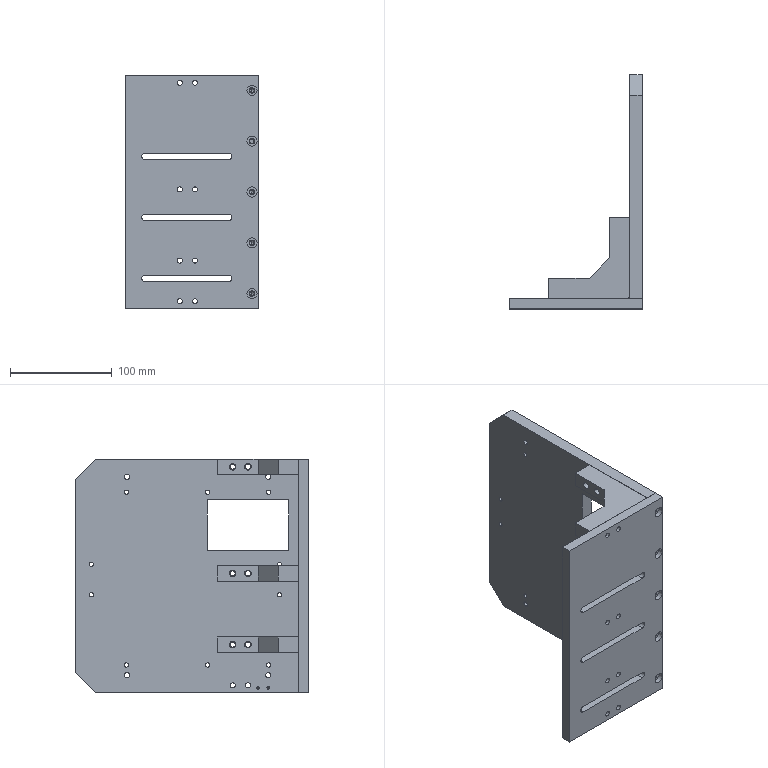Part | SolidWorks | features LocalLPattern 2, ReferencePattern 2 | 5 solids | 198 faces | box 130 x 230 x 230 mm | volume 953540 mm3 | cylinder 127 | plane 59 | cone 12 | commonest cylinder face diameters 5 x40 4.2 x30 6.5 x24 5.5 x10 10 x10 6.6 x9